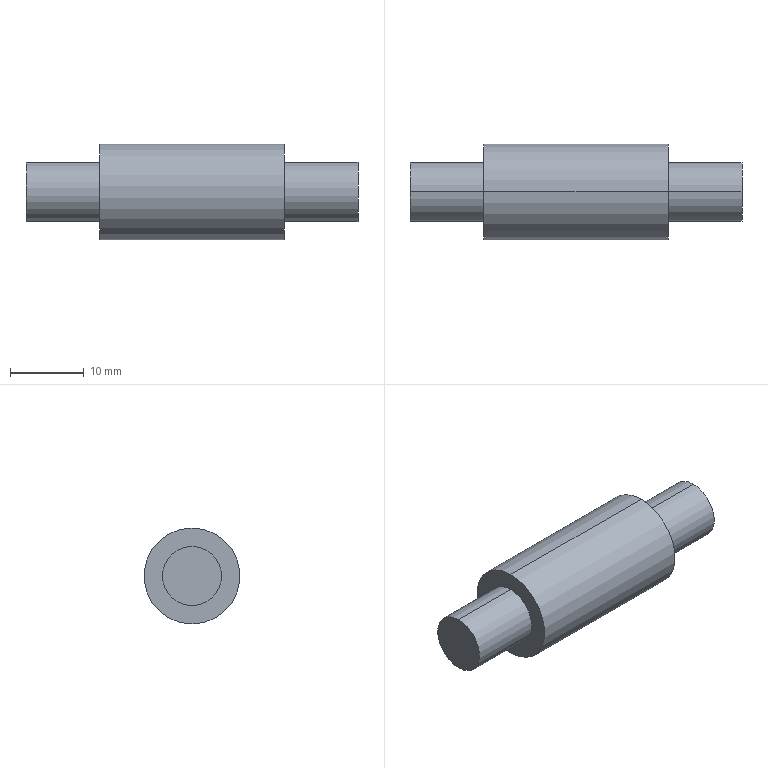Part | SolidWorks | features Extrusion 1, ICE 1, MirrorPattern 1 | 1 solid | 10 faces | box 45 x 13 x 13 mm | volume 4324 mm3 | cylinder 6 | plane 4 | commonest cylinder face diameters 8 x4 13 x2
STEP:
#1=CARTESIAN_POINT('',(-22.5,0.,-4.));
#2=VERTEX_POINT('',#1);
#3=CARTESIAN_POINT('',(-22.5,0.,4.));
#4=VERTEX_POINT('',#3);
#5=CARTESIAN_POINT('',(-22.5,0.,0.));
#6=DIRECTION('',(1.,0.,0.));
#7=DIRECTION('',(0.,0.,-1.));
#8=AXIS2_PLACEMENT_3D('',#5,#6,#7);
#9=CIRCLE('',#8,4.);
#10=EDGE_CURVE('',#2,#4,#9,.T.);
#11=ORIENTED_EDGE('',*,*,#10,.T.);
#12=CARTESIAN_POINT('',(-12.5,0.,4.));
#13=VERTEX_POINT('',#12);
#14=CARTESIAN_POINT('',(-22.5,0.,4.));
#15=DIRECTION('',(1.,0.,0.));
#16=VECTOR('',#15,1000.);
#17=LINE('',#14,#16);
#18=EDGE_CURVE('',#4,#13,#17,.T.);
#19=ORIENTED_EDGE('',*,*,#18,.T.);
#20=CARTESIAN_POINT('',(-12.5,0.,-4.));
#21=VERTEX_POINT('',#20);
#22=CARTESIAN_POINT('',(-12.5,0.,0.));
#23=DIRECTION('',(1.,0.,0.));
#24=DIRECTION('',(0.,0.,-1.));
#25=AXIS2_PLACEMENT_3D('',#22,#23,#24);
#26=CIRCLE('',#25,4.);
#27=EDGE_CURVE('',#21,#13,#26,.T.);
#28=ORIENTED_EDGE('',*,*,#27,.F.);
#29=CARTESIAN_POINT('',(-22.5,0.,-4.));
#30=DIRECTION('',(1.,0.,0.));
#31=VECTOR('',#30,1000.);
#32=LINE('',#29,#31);
#33=EDGE_CURVE('',#2,#21,#32,.T.);
#34=ORIENTED_EDGE('',*,*,#33,.F.);
#35=EDGE_LOOP('',(#11,#19,#28,#34));
#36=FACE_OUTER_BOUND('',#35,.T.);
#37=CARTESIAN_POINT('',(-22.5,0.,0.));
#38=DIRECTION('',(1.,0.,0.));
#39=DIRECTION('',(0.,0.,-1.));
#40=AXIS2_PLACEMENT_3D('',#37,#38,#39);
#41=CYLINDRICAL_SURFACE('',#40,4.);
#42=ADVANCED_FACE('',(#36),#41,.T.);
#43=CARTESIAN_POINT('',(22.5,0.,-4.));
#44=VERTEX_POINT('',#43);
#45=CARTESIAN_POINT('',(22.5,0.,4.));
#46=VERTEX_POINT('',#45);
#47=CARTESIAN_POINT('',(22.5,0.,0.));
#48=DIRECTION('',(1.,0.,0.));
#49=DIRECTION('',(0.,0.,-1.));
#50=AXIS2_PLACEMENT_3D('',#47,#48,#49);
#51=CIRCLE('',#50,4.);
#52=EDGE_CURVE('',#44,#46,#51,.T.);
#53=ORIENTED_EDGE('',*,*,#52,.F.);
#54=CARTESIAN_POINT('',(12.5,0.,-4.));
#55=VERTEX_POINT('',#54);
#56=CARTESIAN_POINT('',(22.5,0.,-4.));
#57=DIRECTION('',(-1.,0.,0.));
#58=VECTOR('',#57,1000.);
#59=LINE('',#56,#58);
#60=EDGE_CURVE('',#44,#55,#59,.T.);
#61=ORIENTED_EDGE('',*,*,#60,.T.);
#62=CARTESIAN_POINT('',(12.5,0.,4.));
#63=VERTEX_POINT('',#62);
#64=CARTESIAN_POINT('',(12.5,0.,0.));
#65=DIRECTION('',(1.,0.,0.));
#66=DIRECTION('',(0.,0.,-1.));
#67=AXIS2_PLACEMENT_3D('',#64,#65,#66);
#68=CIRCLE('',#67,4.);
#69=EDGE_CURVE('',#55,#63,#68,.T.);
#70=ORIENTED_EDGE('',*,*,#69,.T.);
#71=CARTESIAN_POINT('',(22.5,0.,4.));
#72=DIRECTION('',(-1.,0.,0.));
#73=VECTOR('',#72,1000.);
#74=LINE('',#71,#73);
#75=EDGE_CURVE('',#46,#63,#74,.T.);
#76=ORIENTED_EDGE('',*,*,#75,.F.);
#77=EDGE_LOOP('',(#53,#61,#70,#76));
#78=FACE_OUTER_BOUND('',#77,.T.);
#79=CARTESIAN_POINT('',(22.5,0.,0.));
#80=DIRECTION('',(-1.,0.,0.));
#81=DIRECTION('',(0.,0.,1.));
#82=AXIS2_PLACEMENT_3D('',#79,#80,#81);
#83=CYLINDRICAL_SURFACE('',#82,4.);
#84=ADVANCED_FACE('',(#78),#83,.T.);
#85=CARTESIAN_POINT('',(12.5,0.,-6.5));
#86=VERTEX_POINT('',#85);
#87=CARTESIAN_POINT('',(12.5,0.,6.5));
#88=VERTEX_POINT('',#87);
#89=CARTESIAN_POINT('',(12.5,0.,0.));
#90=DIRECTION('',(1.,0.,0.));
#91=DIRECTION('',(0.,0.,-1.));
#92=AXIS2_PLACEMENT_3D('',#89,#90,#91);
#93=CIRCLE('',#92,6.5);
#94=EDGE_CURVE('',#86,#88,#93,.T.);
#95=ORIENTED_EDGE('',*,*,#94,.F.);
#96=CARTESIAN_POINT('',(-12.5,0.,-6.5));
#97=VERTEX_POINT('',#96);
#98=CARTESIAN_POINT('',(12.5,0.,-6.5));
#99=DIRECTION('',(-1.,0.,0.));
#100=VECTOR('',#99,1000.);
#101=LINE('',#98,#100);
#102=EDGE_CURVE('',#86,#97,#101,.T.);
#103=ORIENTED_EDGE('',*,*,#102,.T.);
#104=CARTESIAN_POINT('',(-12.5,0.,6.5));
#105=VERTEX_POINT('',#104);
#106=CARTESIAN_POINT('',(-12.5,0.,0.));
#107=DIRECTION('',(1.,0.,0.));
#108=DIRECTION('',(0.,0.,-1.));
#109=AXIS2_PLACEMENT_3D('',#106,#107,#108);
#110=CIRCLE('',#109,6.5);
#111=EDGE_CURVE('',#97,#105,#110,.T.);
#112=ORIENTED_EDGE('',*,*,#111,.T.);
#113=CARTESIAN_POINT('',(12.5,0.,6.5));
#114=DIRECTION('',(-1.,0.,0.));
#115=VECTOR('',#114,1000.);
#116=LINE('',#113,#115);
#117=EDGE_CURVE('',#88,#105,#116,.T.);
#118=ORIENTED_EDGE('',*,*,#117,.F.);
#119=EDGE_LOOP('',(#95,#103,#112,#118));
#120=FACE_OUTER_BOUND('',#119,.T.);
#121=CARTESIAN_POINT('',(12.5,0.,0.));
#122=DIRECTION('',(-1.,0.,0.));
#123=DIRECTION('',(0.,0.,1.));
#124=AXIS2_PLACEMENT_3D('',#121,#122,#123);
#125=CYLINDRICAL_SURFACE('',#124,6.5);
#126=ADVANCED_FACE('',(#120),#125,.T.);
#127=ORIENTED_EDGE('',*,*,#102,.F.);
#128=CARTESIAN_POINT('',(12.5,0.,0.));
#129=DIRECTION('',(1.,0.,0.));
#130=DIRECTION('',(0.,0.,-1.));
#131=AXIS2_PLACEMENT_3D('',#128,#129,#130);
#132=CIRCLE('',#131,6.5);
#133=EDGE_CURVE('',#88,#86,#132,.T.);
#134=ORIENTED_EDGE('',*,*,#133,.F.);
#135=ORIENTED_EDGE('',*,*,#117,.T.);
#136=CARTESIAN_POINT('',(-12.5,0.,0.));
#137=DIRECTION('',(1.,0.,0.));
#138=DIRECTION('',(0.,0.,-1.));
#139=AXIS2_PLACEMENT_3D('',#136,#137,#138);
#140=CIRCLE('',#139,6.5);
#141=EDGE_CURVE('',#105,#97,#140,.T.);
#142=ORIENTED_EDGE('',*,*,#141,.T.);
#143=EDGE_LOOP('',(#127,#134,#135,#142));
#144=FACE_OUTER_BOUND('',#143,.T.);
#145=CARTESIAN_POINT('',(12.5,0.,0.));
#146=DIRECTION('',(-1.,0.,0.));
#147=DIRECTION('',(0.,0.,1.));
#148=AXIS2_PLACEMENT_3D('',#145,#146,#147);
#149=CYLINDRICAL_SURFACE('',#148,6.5);
#150=ADVANCED_FACE('',(#144),#149,.T.);
#151=CARTESIAN_POINT('',(12.5,0.,0.));
#152=DIRECTION('',(1.,0.,0.));
#153=DIRECTION('',(0.,0.,-1.));
#154=AXIS2_PLACEMENT_3D('',#151,#152,#153);
#155=CIRCLE('',#154,4.);
#156=EDGE_CURVE('',#63,#55,#155,.T.);
#157=ORIENTED_EDGE('',*,*,#156,.F.);
#158=ORIENTED_EDGE('',*,*,#69,.F.);
#159=EDGE_LOOP('',(#157,#158));
#160=FACE_BOUND('',#159,.T.);
#161=ORIENTED_EDGE('',*,*,#133,.T.);
#162=ORIENTED_EDGE('',*,*,#94,.T.);
#163=EDGE_LOOP('',(#161,#162));
#164=FACE_OUTER_BOUND('',#163,.T.);
#165=CARTESIAN_POINT('',(12.5,0.,0.));
#166=DIRECTION('',(1.,0.,0.));
#167=DIRECTION('',(0.,0.,-1.));
#168=AXIS2_PLACEMENT_3D('',#165,#166,#167);
#169=PLANE('',#168);
#170=ADVANCED_FACE('',(#160,#164),#169,.T.);
#171=ORIENTED_EDGE('',*,*,#27,.T.);
#172=CARTESIAN_POINT('',(-12.5,0.,0.));
#173=DIRECTION('',(1.,0.,0.));
#174=DIRECTION('',(0.,0.,-1.));
#175=AXIS2_PLACEMENT_3D('',#172,#173,#174);
#176=CIRCLE('',#175,4.);
#177=EDGE_CURVE('',#13,#21,#176,.T.);
#178=ORIENTED_EDGE('',*,*,#177,.T.);
#179=EDGE_LOOP('',(#171,#178));
#180=FACE_BOUND('',#179,.T.);
#181=ORIENTED_EDGE('',*,*,#141,.F.);
#182=ORIENTED_EDGE('',*,*,#111,.F.);
#183=EDGE_LOOP('',(#181,#182));
#184=FACE_OUTER_BOUND('',#183,.T.);
#185=CARTESIAN_POINT('',(-12.5,0.,0.));
#186=DIRECTION('',(1.,0.,0.));
#187=DIRECTION('',(0.,0.,-1.));
#188=AXIS2_PLACEMENT_3D('',#185,#186,#187);
#189=PLANE('',#188);
#190=ADVANCED_FACE('',(#180,#184),#189,.F.);
#191=ORIENTED_EDGE('',*,*,#60,.F.);
#192=CARTESIAN_POINT('',(22.5,0.,0.));
#193=DIRECTION('',(1.,0.,0.));
#194=DIRECTION('',(0.,0.,-1.));
#195=AXIS2_PLACEMENT_3D('',#192,#193,#194);
#196=CIRCLE('',#195,4.);
#197=EDGE_CURVE('',#46,#44,#196,.T.);
#198=ORIENTED_EDGE('',*,*,#197,.F.);
#199=ORIENTED_EDGE('',*,*,#75,.T.);
#200=ORIENTED_EDGE('',*,*,#156,.T.);
#201=EDGE_LOOP('',(#191,#198,#199,#200));
#202=FACE_OUTER_BOUND('',#201,.T.);
#203=CARTESIAN_POINT('',(22.5,0.,0.));
#204=DIRECTION('',(-1.,0.,0.));
#205=DIRECTION('',(0.,0.,1.));
#206=AXIS2_PLACEMENT_3D('',#203,#204,#205);
#207=CYLINDRICAL_SURFACE('',#206,4.);
#208=ADVANCED_FACE('',(#202),#207,.T.);
#209=ORIENTED_EDGE('',*,*,#197,.T.);
#210=ORIENTED_EDGE('',*,*,#52,.T.);
#211=EDGE_LOOP('',(#209,#210));
#212=FACE_OUTER_BOUND('',#211,.T.);
#213=CARTESIAN_POINT('',(22.5,0.,0.));
#214=DIRECTION('',(1.,0.,0.));
#215=DIRECTION('',(0.,0.,-1.));
#216=AXIS2_PLACEMENT_3D('',#213,#214,#215);
#217=PLANE('',#216);
#218=ADVANCED_FACE('',(#212),#217,.T.);
#219=ORIENTED_EDGE('',*,*,#18,.F.);
#220=CARTESIAN_POINT('',(-22.5,0.,0.));
#221=DIRECTION('',(1.,0.,0.));
#222=DIRECTION('',(0.,0.,-1.));
#223=AXIS2_PLACEMENT_3D('',#220,#221,#222);
#224=CIRCLE('',#223,4.);
#225=EDGE_CURVE('',#4,#2,#224,.T.);
#226=ORIENTED_EDGE('',*,*,#225,.T.);
#227=ORIENTED_EDGE('',*,*,#33,.T.);
#228=ORIENTED_EDGE('',*,*,#177,.F.);
#229=EDGE_LOOP('',(#219,#226,#227,#228));
#230=FACE_OUTER_BOUND('',#229,.T.);
#231=CARTESIAN_POINT('',(-22.5,0.,0.));
#232=DIRECTION('',(1.,0.,0.));
#233=DIRECTION('',(0.,0.,-1.));
#234=AXIS2_PLACEMENT_3D('',#231,#232,#233);
#235=CYLINDRICAL_SURFACE('',#234,4.);
#236=ADVANCED_FACE('',(#230),#235,.T.);
#237=ORIENTED_EDGE('',*,*,#10,.F.);
#238=ORIENTED_EDGE('',*,*,#225,.F.);
#239=EDGE_LOOP('',(#237,#238));
#240=FACE_OUTER_BOUND('',#239,.T.);
#241=CARTESIAN_POINT('',(-22.5,0.,0.));
#242=DIRECTION('',(-1.,0.,0.));
#243=DIRECTION('',(0.,0.,-1.));
#244=AXIS2_PLACEMENT_3D('',#241,#242,#243);
#245=PLANE('',#244);
#246=ADVANCED_FACE('',(#240),#245,.T.);
#247=CLOSED_SHELL('',(#42,#84,#126,#150,#170,#190,#208,#218,#236,#246));
#248=MANIFOLD_SOLID_BREP('',#247);
#249=CARTESIAN_POINT('',(0.,0.,0.));
#250=DIRECTION('',(0.,0.,1.));
#251=DIRECTION('',(1.,0.,0.));
#252=AXIS2_PLACEMENT_3D('',#249,#250,#251);
#253=(LENGTH_UNIT()NAMED_UNIT(*)SI_UNIT(.MILLI.,.METRE.));
#254=UNCERTAINTY_MEASURE_WITH_UNIT(LENGTH_MEASURE(0.00001),#253,'','');
#255=(NAMED_UNIT(*)PLANE_ANGLE_UNIT()SI_UNIT($,.RADIAN.));
#256=(NAMED_UNIT(*)SI_UNIT($,.STERADIAN.)SOLID_ANGLE_UNIT());
#257=(GEOMETRIC_REPRESENTATION_CONTEXT(3)GLOBAL_UNCERTAINTY_ASSIGNED_CONTEXT((#254))GLOBAL_UNIT_ASSIGNED_CONTEXT((#253,#255,#256))REPRESENTATION_CONTEXT('',''));
#258=ADVANCED_BREP_SHAPE_REPRESENTATION('',(#248,#252),#257);